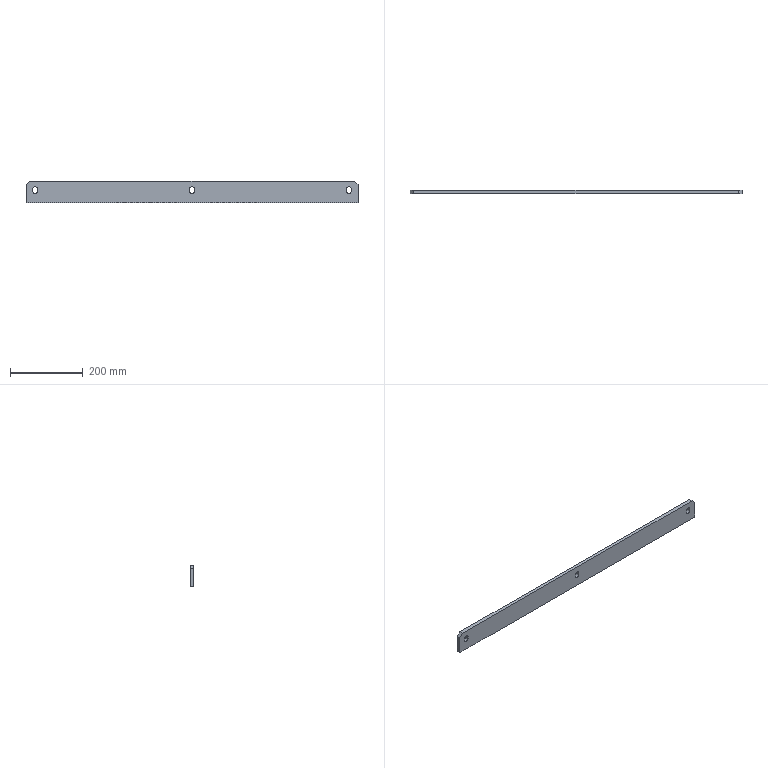Part | NX | features solid 2 | 1 solid | 20 faces | box 910 x 10 x 60 mm | volume 538678 mm3 | plane 14 | cylinder 6 | commonest cylinder face diameters 13 x6
STEP:
#1=CARTESIAN_POINT('',(570.,10.,-50.));
#2=VERTEX_POINT('',#1);
#3=CARTESIAN_POINT('',(580.,10.,-60.));
#4=VERTEX_POINT('',#3);
#5=CARTESIAN_POINT('',(580.,10.,-60.));
#6=DIRECTION('',(0.7071,0.,-0.7071));
#7=VECTOR('',#6,1000.);
#8=LINE('',#5,#7);
#9=EDGE_CURVE('',#2,#4,#8,.T.);
#10=ORIENTED_EDGE('',*,*,#9,.F.);
#11=CARTESIAN_POINT('',(570.,0.,-50.));
#12=VERTEX_POINT('',#11);
#13=CARTESIAN_POINT('',(570.,0.,-50.));
#14=DIRECTION('',(0.,1.,0.));
#15=VECTOR('',#14,1000.);
#16=LINE('',#13,#15);
#17=EDGE_CURVE('',#12,#2,#16,.T.);
#18=ORIENTED_EDGE('',*,*,#17,.F.);
#19=CARTESIAN_POINT('',(580.,0.,-60.));
#20=VERTEX_POINT('',#19);
#21=CARTESIAN_POINT('',(155.,0.,365.));
#22=DIRECTION('',(-0.7071,0.,0.7071));
#23=VECTOR('',#22,1000.);
#24=LINE('',#21,#23);
#25=EDGE_CURVE('',#20,#12,#24,.T.);
#26=ORIENTED_EDGE('',*,*,#25,.F.);
#27=CARTESIAN_POINT('',(580.,10.,-60.));
#28=DIRECTION('',(0.,-1.,0.));
#29=VECTOR('',#28,1000.);
#30=LINE('',#27,#29);
#31=EDGE_CURVE('',#4,#20,#30,.T.);
#32=ORIENTED_EDGE('',*,*,#31,.F.);
#33=EDGE_LOOP('',(#10,#18,#26,#32));
#34=FACE_BOUND('',#33,.T.);
#35=CARTESIAN_POINT('',(580.,10.,-60.));
#36=DIRECTION('',(-0.7071,0.,-0.7071));
#37=DIRECTION('',(-0.7071,0.,0.7071));
#38=AXIS2_PLACEMENT_3D('',#35,#36,#37);
#39=PLANE('',#38);
#40=ADVANCED_FACE('',(#34),#39,.F.);
#41=CARTESIAN_POINT('',(-330.,10.,-60.));
#42=VERTEX_POINT('',#41);
#43=CARTESIAN_POINT('',(-320.,10.,-50.));
#44=VERTEX_POINT('',#43);
#45=CARTESIAN_POINT('',(-320.,10.,-50.));
#46=DIRECTION('',(0.7071,0.,0.7071));
#47=VECTOR('',#46,1000.);
#48=LINE('',#45,#47);
#49=EDGE_CURVE('',#42,#44,#48,.T.);
#50=ORIENTED_EDGE('',*,*,#49,.F.);
#51=CARTESIAN_POINT('',(-330.,0.,-60.));
#52=VERTEX_POINT('',#51);
#53=CARTESIAN_POINT('',(-330.,10.,-60.));
#54=DIRECTION('',(0.,1.,0.));
#55=VECTOR('',#54,1000.);
#56=LINE('',#53,#55);
#57=EDGE_CURVE('',#52,#42,#56,.T.);
#58=ORIENTED_EDGE('',*,*,#57,.F.);
#59=CARTESIAN_POINT('',(-320.,0.,-50.));
#60=VERTEX_POINT('',#59);
#61=CARTESIAN_POINT('',(-360.,0.,-90.));
#62=DIRECTION('',(-0.7071,0.,-0.7071));
#63=VECTOR('',#62,1000.);
#64=LINE('',#61,#63);
#65=EDGE_CURVE('',#60,#52,#64,.T.);
#66=ORIENTED_EDGE('',*,*,#65,.F.);
#67=CARTESIAN_POINT('',(-320.,0.,-50.));
#68=DIRECTION('',(0.,-1.,0.));
#69=VECTOR('',#68,1000.);
#70=LINE('',#67,#69);
#71=EDGE_CURVE('',#44,#60,#70,.T.);
#72=ORIENTED_EDGE('',*,*,#71,.F.);
#73=EDGE_LOOP('',(#50,#58,#66,#72));
#74=FACE_BOUND('',#73,.T.);
#75=CARTESIAN_POINT('',(-320.,0.,-50.));
#76=DIRECTION('',(0.7071,0.,-0.7071));
#77=DIRECTION('',(0.,-1.,0.));
#78=AXIS2_PLACEMENT_3D('',#75,#76,#77);
#79=PLANE('',#78);
#80=ADVANCED_FACE('',(#74),#79,.F.);
#81=CARTESIAN_POINT('',(580.,10.,-110.));
#82=VERTEX_POINT('',#81);
#83=CARTESIAN_POINT('',(580.,10.,-120.));
#84=DIRECTION('',(0.,0.,1.));
#85=VECTOR('',#84,1000.);
#86=LINE('',#83,#85);
#87=EDGE_CURVE('',#82,#4,#86,.T.);
#88=ORIENTED_EDGE('',*,*,#87,.T.);
#89=ORIENTED_EDGE('',*,*,#31,.T.);
#90=CARTESIAN_POINT('',(580.,0.,-110.));
#91=VERTEX_POINT('',#90);
#92=CARTESIAN_POINT('',(580.,0.,-120.));
#93=DIRECTION('',(0.,0.,1.));
#94=VECTOR('',#93,1000.);
#95=LINE('',#92,#94);
#96=EDGE_CURVE('',#91,#20,#95,.T.);
#97=ORIENTED_EDGE('',*,*,#96,.F.);
#98=CARTESIAN_POINT('',(580.,10.,-110.));
#99=DIRECTION('',(0.,1.,0.));
#100=VECTOR('',#99,1000.);
#101=LINE('',#98,#100);
#102=EDGE_CURVE('',#91,#82,#101,.T.);
#103=ORIENTED_EDGE('',*,*,#102,.T.);
#104=EDGE_LOOP('',(#88,#89,#97,#103));
#105=FACE_BOUND('',#104,.T.);
#106=CARTESIAN_POINT('',(580.,10.,-120.));
#107=DIRECTION('',(-1.,0.,0.));
#108=DIRECTION('',(0.,0.,1.));
#109=AXIS2_PLACEMENT_3D('',#106,#107,#108);
#110=PLANE('',#109);
#111=ADVANCED_FACE('',(#105),#110,.F.);
#112=CARTESIAN_POINT('',(561.5,0.,-78.));
#113=VERTEX_POINT('',#112);
#114=CARTESIAN_POINT('',(561.5,10.,-78.));
#115=VERTEX_POINT('',#114);
#116=CARTESIAN_POINT('',(561.5,5.,-78.));
#117=DIRECTION('',(0.,1.,0.));
#118=VECTOR('',#117,1000.);
#119=LINE('',#116,#118);
#120=EDGE_CURVE('',#113,#115,#119,.T.);
#121=ORIENTED_EDGE('',*,*,#120,.T.);
#122=CARTESIAN_POINT('',(548.5,10.,-78.));
#123=VERTEX_POINT('',#122);
#124=CARTESIAN_POINT('',(555.,10.,-78.));
#125=DIRECTION('',(0.,1.,0.));
#126=DIRECTION('',(1.,0.,0.));
#127=AXIS2_PLACEMENT_3D('',#124,#125,#126);
#128=CIRCLE('',#127,6.5);
#129=EDGE_CURVE('',#115,#123,#128,.T.);
#130=ORIENTED_EDGE('',*,*,#129,.T.);
#131=CARTESIAN_POINT('',(548.5,0.,-78.));
#132=VERTEX_POINT('',#131);
#133=CARTESIAN_POINT('',(548.5,5.,-78.));
#134=DIRECTION('',(0.,-1.,0.));
#135=VECTOR('',#134,1000.);
#136=LINE('',#133,#135);
#137=EDGE_CURVE('',#123,#132,#136,.T.);
#138=ORIENTED_EDGE('',*,*,#137,.T.);
#139=CARTESIAN_POINT('',(555.,0.,-78.));
#140=DIRECTION('',(0.,1.,0.));
#141=DIRECTION('',(1.,0.,0.));
#142=AXIS2_PLACEMENT_3D('',#139,#140,#141);
#143=CIRCLE('',#142,6.5);
#144=EDGE_CURVE('',#113,#132,#143,.T.);
#145=ORIENTED_EDGE('',*,*,#144,.F.);
#146=EDGE_LOOP('',(#121,#130,#138,#145));
#147=FACE_BOUND('',#146,.T.);
#148=CARTESIAN_POINT('',(555.,5.,-78.));
#149=DIRECTION('',(0.,-1.,0.));
#150=DIRECTION('',(1.,0.,0.));
#151=AXIS2_PLACEMENT_3D('',#148,#149,#150);
#152=CYLINDRICAL_SURFACE('',#151,6.5);
#153=ADVANCED_FACE('',(#147),#152,.F.);
#154=ORIENTED_EDGE('',*,*,#137,.F.);
#155=CARTESIAN_POINT('',(548.5,10.,-72.));
#156=VERTEX_POINT('',#155);
#157=CARTESIAN_POINT('',(548.5,10.,-78.));
#158=DIRECTION('',(0.,0.,1.));
#159=VECTOR('',#158,1000.);
#160=LINE('',#157,#159);
#161=EDGE_CURVE('',#123,#156,#160,.T.);
#162=ORIENTED_EDGE('',*,*,#161,.T.);
#163=CARTESIAN_POINT('',(548.5,0.,-72.));
#164=VERTEX_POINT('',#163);
#165=CARTESIAN_POINT('',(548.5,10.,-72.));
#166=DIRECTION('',(0.,-1.,0.));
#167=VECTOR('',#166,1000.);
#168=LINE('',#165,#167);
#169=EDGE_CURVE('',#156,#164,#168,.T.);
#170=ORIENTED_EDGE('',*,*,#169,.T.);
#171=CARTESIAN_POINT('',(548.5,0.,-78.));
#172=DIRECTION('',(0.,0.,1.));
#173=VECTOR('',#172,1000.);
#174=LINE('',#171,#173);
#175=EDGE_CURVE('',#132,#164,#174,.T.);
#176=ORIENTED_EDGE('',*,*,#175,.F.);
#177=EDGE_LOOP('',(#154,#162,#170,#176));
#178=FACE_BOUND('',#177,.T.);
#179=CARTESIAN_POINT('',(548.5,10.,-78.));
#180=DIRECTION('',(-1.,0.,0.));
#181=DIRECTION('',(0.,0.,1.));
#182=AXIS2_PLACEMENT_3D('',#179,#180,#181);
#183=PLANE('',#182);
#184=ADVANCED_FACE('',(#178),#183,.F.);
#185=ORIENTED_EDGE('',*,*,#169,.F.);
#186=CARTESIAN_POINT('',(561.5,10.,-72.));
#187=VERTEX_POINT('',#186);
#188=CARTESIAN_POINT('',(555.,10.,-72.));
#189=DIRECTION('',(0.,1.,0.));
#190=DIRECTION('',(1.,0.,0.));
#191=AXIS2_PLACEMENT_3D('',#188,#189,#190);
#192=CIRCLE('',#191,6.5);
#193=EDGE_CURVE('',#156,#187,#192,.T.);
#194=ORIENTED_EDGE('',*,*,#193,.T.);
#195=CARTESIAN_POINT('',(561.5,0.,-72.));
#196=VERTEX_POINT('',#195);
#197=CARTESIAN_POINT('',(561.5,5.,-72.));
#198=DIRECTION('',(0.,-1.,0.));
#199=VECTOR('',#198,1000.);
#200=LINE('',#197,#199);
#201=EDGE_CURVE('',#187,#196,#200,.T.);
#202=ORIENTED_EDGE('',*,*,#201,.T.);
#203=CARTESIAN_POINT('',(555.,0.,-72.));
#204=DIRECTION('',(0.,1.,0.));
#205=DIRECTION('',(1.,0.,0.));
#206=AXIS2_PLACEMENT_3D('',#203,#204,#205);
#207=CIRCLE('',#206,6.5);
#208=EDGE_CURVE('',#164,#196,#207,.T.);
#209=ORIENTED_EDGE('',*,*,#208,.F.);
#210=EDGE_LOOP('',(#185,#194,#202,#209));
#211=FACE_BOUND('',#210,.T.);
#212=CARTESIAN_POINT('',(555.,5.,-72.));
#213=DIRECTION('',(0.,-1.,0.));
#214=DIRECTION('',(1.,0.,0.));
#215=AXIS2_PLACEMENT_3D('',#212,#213,#214);
#216=CYLINDRICAL_SURFACE('',#215,6.5);
#217=ADVANCED_FACE('',(#211),#216,.F.);
#218=ORIENTED_EDGE('',*,*,#201,.F.);
#219=CARTESIAN_POINT('',(561.5,10.,-78.));
#220=DIRECTION('',(0.,0.,-1.));
#221=VECTOR('',#220,1000.);
#222=LINE('',#219,#221);
#223=EDGE_CURVE('',#187,#115,#222,.T.);
#224=ORIENTED_EDGE('',*,*,#223,.T.);
#225=ORIENTED_EDGE('',*,*,#120,.F.);
#226=CARTESIAN_POINT('',(561.5,0.,-78.));
#227=DIRECTION('',(0.,0.,-1.));
#228=VECTOR('',#227,1000.);
#229=LINE('',#226,#228);
#230=EDGE_CURVE('',#196,#113,#229,.T.);
#231=ORIENTED_EDGE('',*,*,#230,.F.);
#232=EDGE_LOOP('',(#218,#224,#225,#231));
#233=FACE_BOUND('',#232,.T.);
#234=CARTESIAN_POINT('',(561.5,0.,-78.));
#235=DIRECTION('',(1.,0.,0.));
#236=DIRECTION('',(0.,-1.,0.));
#237=AXIS2_PLACEMENT_3D('',#234,#235,#236);
#238=PLANE('',#237);
#239=ADVANCED_FACE('',(#233),#238,.F.);
#240=CARTESIAN_POINT('',(131.5,0.,-78.));
#241=VERTEX_POINT('',#240);
#242=CARTESIAN_POINT('',(131.5,10.,-78.));
#243=VERTEX_POINT('',#242);
#244=CARTESIAN_POINT('',(131.5,5.,-78.));
#245=DIRECTION('',(0.,1.,0.));
#246=VECTOR('',#245,1000.);
#247=LINE('',#244,#246);
#248=EDGE_CURVE('',#241,#243,#247,.T.);
#249=ORIENTED_EDGE('',*,*,#248,.T.);
#250=CARTESIAN_POINT('',(118.5,10.,-78.));
#251=VERTEX_POINT('',#250);
#252=CARTESIAN_POINT('',(125.,10.,-78.));
#253=DIRECTION('',(0.,1.,0.));
#254=DIRECTION('',(1.,0.,0.));
#255=AXIS2_PLACEMENT_3D('',#252,#253,#254);
#256=CIRCLE('',#255,6.5);
#257=EDGE_CURVE('',#243,#251,#256,.T.);
#258=ORIENTED_EDGE('',*,*,#257,.T.);
#259=CARTESIAN_POINT('',(118.5,0.,-78.));
#260=VERTEX_POINT('',#259);
#261=CARTESIAN_POINT('',(118.5,5.,-78.));
#262=DIRECTION('',(0.,-1.,0.));
#263=VECTOR('',#262,1000.);
#264=LINE('',#261,#263);
#265=EDGE_CURVE('',#251,#260,#264,.T.);
#266=ORIENTED_EDGE('',*,*,#265,.T.);
#267=CARTESIAN_POINT('',(125.,0.,-78.));
#268=DIRECTION('',(0.,1.,0.));
#269=DIRECTION('',(1.,0.,0.));
#270=AXIS2_PLACEMENT_3D('',#267,#268,#269);
#271=CIRCLE('',#270,6.5);
#272=EDGE_CURVE('',#241,#260,#271,.T.);
#273=ORIENTED_EDGE('',*,*,#272,.F.);
#274=EDGE_LOOP('',(#249,#258,#266,#273));
#275=FACE_BOUND('',#274,.T.);
#276=CARTESIAN_POINT('',(125.,5.,-78.));
#277=DIRECTION('',(0.,-1.,0.));
#278=DIRECTION('',(1.,0.,0.));
#279=AXIS2_PLACEMENT_3D('',#276,#277,#278);
#280=CYLINDRICAL_SURFACE('',#279,6.5);
#281=ADVANCED_FACE('',(#275),#280,.F.);
#282=ORIENTED_EDGE('',*,*,#265,.F.);
#283=CARTESIAN_POINT('',(118.5,10.,-72.));
#284=VERTEX_POINT('',#283);
#285=CARTESIAN_POINT('',(118.5,10.,-78.));
#286=DIRECTION('',(0.,0.,1.));
#287=VECTOR('',#286,1000.);
#288=LINE('',#285,#287);
#289=EDGE_CURVE('',#251,#284,#288,.T.);
#290=ORIENTED_EDGE('',*,*,#289,.T.);
#291=CARTESIAN_POINT('',(118.5,0.,-72.));
#292=VERTEX_POINT('',#291);
#293=CARTESIAN_POINT('',(118.5,10.,-72.));
#294=DIRECTION('',(0.,-1.,0.));
#295=VECTOR('',#294,1000.);
#296=LINE('',#293,#295);
#297=EDGE_CURVE('',#284,#292,#296,.T.);
#298=ORIENTED_EDGE('',*,*,#297,.T.);
#299=CARTESIAN_POINT('',(118.5,0.,-78.));
#300=DIRECTION('',(0.,0.,1.));
#301=VECTOR('',#300,1000.);
#302=LINE('',#299,#301);
#303=EDGE_CURVE('',#260,#292,#302,.T.);
#304=ORIENTED_EDGE('',*,*,#303,.F.);
#305=EDGE_LOOP('',(#282,#290,#298,#304));
#306=FACE_BOUND('',#305,.T.);
#307=CARTESIAN_POINT('',(118.5,10.,-78.));
#308=DIRECTION('',(-1.,0.,0.));
#309=DIRECTION('',(0.,0.,1.));
#310=AXIS2_PLACEMENT_3D('',#307,#308,#309);
#311=PLANE('',#310);
#312=ADVANCED_FACE('',(#306),#311,.F.);
#313=ORIENTED_EDGE('',*,*,#297,.F.);
#314=CARTESIAN_POINT('',(131.5,10.,-72.));
#315=VERTEX_POINT('',#314);
#316=CARTESIAN_POINT('',(125.,10.,-72.));
#317=DIRECTION('',(0.,1.,0.));
#318=DIRECTION('',(1.,0.,0.));
#319=AXIS2_PLACEMENT_3D('',#316,#317,#318);
#320=CIRCLE('',#319,6.5);
#321=EDGE_CURVE('',#284,#315,#320,.T.);
#322=ORIENTED_EDGE('',*,*,#321,.T.);
#323=CARTESIAN_POINT('',(131.5,0.,-72.));
#324=VERTEX_POINT('',#323);
#325=CARTESIAN_POINT('',(131.5,5.,-72.));
#326=DIRECTION('',(0.,-1.,0.));
#327=VECTOR('',#326,1000.);
#328=LINE('',#325,#327);
#329=EDGE_CURVE('',#315,#324,#328,.T.);
#330=ORIENTED_EDGE('',*,*,#329,.T.);
#331=CARTESIAN_POINT('',(125.,0.,-72.));
#332=DIRECTION('',(0.,1.,0.));
#333=DIRECTION('',(1.,0.,0.));
#334=AXIS2_PLACEMENT_3D('',#331,#332,#333);
#335=CIRCLE('',#334,6.5);
#336=EDGE_CURVE('',#292,#324,#335,.T.);
#337=ORIENTED_EDGE('',*,*,#336,.F.);
#338=EDGE_LOOP('',(#313,#322,#330,#337));
#339=FACE_BOUND('',#338,.T.);
#340=CARTESIAN_POINT('',(125.,5.,-72.));
#341=DIRECTION('',(0.,-1.,0.));
#342=DIRECTION('',(1.,0.,0.));
#343=AXIS2_PLACEMENT_3D('',#340,#341,#342);
#344=CYLINDRICAL_SURFACE('',#343,6.5);
#345=ADVANCED_FACE('',(#339),#344,.F.);
#346=ORIENTED_EDGE('',*,*,#329,.F.);
#347=CARTESIAN_POINT('',(131.5,10.,-78.));
#348=DIRECTION('',(0.,0.,-1.));
#349=VECTOR('',#348,1000.);
#350=LINE('',#347,#349);
#351=EDGE_CURVE('',#315,#243,#350,.T.);
#352=ORIENTED_EDGE('',*,*,#351,.T.);
#353=ORIENTED_EDGE('',*,*,#248,.F.);
#354=CARTESIAN_POINT('',(131.5,0.,-78.));
#355=DIRECTION('',(0.,0.,-1.));
#356=VECTOR('',#355,1000.);
#357=LINE('',#354,#356);
#358=EDGE_CURVE('',#324,#241,#357,.T.);
#359=ORIENTED_EDGE('',*,*,#358,.F.);
#360=EDGE_LOOP('',(#346,#352,#353,#359));
#361=FACE_BOUND('',#360,.T.);
#362=CARTESIAN_POINT('',(131.5,0.,-78.));
#363=DIRECTION('',(1.,0.,0.));
#364=DIRECTION('',(0.,-1.,0.));
#365=AXIS2_PLACEMENT_3D('',#362,#363,#364);
#366=PLANE('',#365);
#367=ADVANCED_FACE('',(#361),#366,.F.);
#368=CARTESIAN_POINT('',(-298.5,0.,-78.));
#369=VERTEX_POINT('',#368);
#370=CARTESIAN_POINT('',(-298.5,10.,-78.));
#371=VERTEX_POINT('',#370);
#372=CARTESIAN_POINT('',(-298.5,5.,-78.));
#373=DIRECTION('',(0.,1.,0.));
#374=VECTOR('',#373,1000.);
#375=LINE('',#372,#374);
#376=EDGE_CURVE('',#369,#371,#375,.T.);
#377=ORIENTED_EDGE('',*,*,#376,.T.);
#378=CARTESIAN_POINT('',(-311.5,10.,-78.));
#379=VERTEX_POINT('',#378);
#380=CARTESIAN_POINT('',(-305.,10.,-78.));
#381=DIRECTION('',(0.,1.,0.));
#382=DIRECTION('',(1.,0.,0.));
#383=AXIS2_PLACEMENT_3D('',#380,#381,#382);
#384=CIRCLE('',#383,6.5);
#385=EDGE_CURVE('',#371,#379,#384,.T.);
#386=ORIENTED_EDGE('',*,*,#385,.T.);
#387=CARTESIAN_POINT('',(-311.5,0.,-78.));
#388=VERTEX_POINT('',#387);
#389=CARTESIAN_POINT('',(-311.5,5.,-78.));
#390=DIRECTION('',(0.,-1.,0.));
#391=VECTOR('',#390,1000.);
#392=LINE('',#389,#391);
#393=EDGE_CURVE('',#379,#388,#392,.T.);
#394=ORIENTED_EDGE('',*,*,#393,.T.);
#395=CARTESIAN_POINT('',(-305.,0.,-78.));
#396=DIRECTION('',(0.,1.,0.));
#397=DIRECTION('',(1.,0.,0.));
#398=AXIS2_PLACEMENT_3D('',#395,#396,#397);
#399=CIRCLE('',#398,6.5);
#400=EDGE_CURVE('',#369,#388,#399,.T.);
#401=ORIENTED_EDGE('',*,*,#400,.F.);
#402=EDGE_LOOP('',(#377,#386,#394,#401));
#403=FACE_BOUND('',#402,.T.);
#404=CARTESIAN_POINT('',(-305.,5.,-78.));
#405=DIRECTION('',(0.,-1.,0.));
#406=DIRECTION('',(1.,0.,0.));
#407=AXIS2_PLACEMENT_3D('',#404,#405,#406);
#408=CYLINDRICAL_SURFACE('',#407,6.5);
#409=ADVANCED_FACE('',(#403),#408,.F.);
#410=ORIENTED_EDGE('',*,*,#393,.F.);
#411=CARTESIAN_POINT('',(-311.5,10.,-72.));
#412=VERTEX_POINT('',#411);
#413=CARTESIAN_POINT('',(-311.5,10.,-78.));
#414=DIRECTION('',(0.,0.,1.));
#415=VECTOR('',#414,1000.);
#416=LINE('',#413,#415);
#417=EDGE_CURVE('',#379,#412,#416,.T.);
#418=ORIENTED_EDGE('',*,*,#417,.T.);
#419=CARTESIAN_POINT('',(-311.5,0.,-72.));
#420=VERTEX_POINT('',#419);
#421=CARTESIAN_POINT('',(-311.5,10.,-72.));
#422=DIRECTION('',(0.,-1.,0.));
#423=VECTOR('',#422,1000.);
#424=LINE('',#421,#423);
#425=EDGE_CURVE('',#412,#420,#424,.T.);
#426=ORIENTED_EDGE('',*,*,#425,.T.);
#427=CARTESIAN_POINT('',(-311.5,0.,-78.));
#428=DIRECTION('',(0.,0.,1.));
#429=VECTOR('',#428,1000.);
#430=LINE('',#427,#429);
#431=EDGE_CURVE('',#388,#420,#430,.T.);
#432=ORIENTED_EDGE('',*,*,#431,.F.);
#433=EDGE_LOOP('',(#410,#418,#426,#432));
#434=FACE_BOUND('',#433,.T.);
#435=CARTESIAN_POINT('',(-311.5,10.,-78.));
#436=DIRECTION('',(-1.,0.,0.));
#437=DIRECTION('',(0.,0.,1.));
#438=AXIS2_PLACEMENT_3D('',#435,#436,#437);
#439=PLANE('',#438);
#440=ADVANCED_FACE('',(#434),#439,.F.);
#441=ORIENTED_EDGE('',*,*,#425,.F.);
#442=CARTESIAN_POINT('',(-298.5,10.,-72.));
#443=VERTEX_POINT('',#442);
#444=CARTESIAN_POINT('',(-305.,10.,-72.));
#445=DIRECTION('',(0.,1.,0.));
#446=DIRECTION('',(1.,0.,0.));
#447=AXIS2_PLACEMENT_3D('',#444,#445,#446);
#448=CIRCLE('',#447,6.5);
#449=EDGE_CURVE('',#412,#443,#448,.T.);
#450=ORIENTED_EDGE('',*,*,#449,.T.);
#451=CARTESIAN_POINT('',(-298.5,0.,-72.));
#452=VERTEX_POINT('',#451);
#453=CARTESIAN_POINT('',(-298.5,5.,-72.));
#454=DIRECTION('',(0.,-1.,0.));
#455=VECTOR('',#454,1000.);
#456=LINE('',#453,#455);
#457=EDGE_CURVE('',#443,#452,#456,.T.);
#458=ORIENTED_EDGE('',*,*,#457,.T.);
#459=CARTESIAN_POINT('',(-305.,0.,-72.));
#460=DIRECTION('',(0.,1.,0.));
#461=DIRECTION('',(1.,0.,0.));
#462=AXIS2_PLACEMENT_3D('',#459,#460,#461);
#463=CIRCLE('',#462,6.5);
#464=EDGE_CURVE('',#420,#452,#463,.T.);
#465=ORIENTED_EDGE('',*,*,#464,.F.);
#466=EDGE_LOOP('',(#441,#450,#458,#465));
#467=FACE_BOUND('',#466,.T.);
#468=CARTESIAN_POINT('',(-305.,5.,-72.));
#469=DIRECTION('',(0.,-1.,0.));
#470=DIRECTION('',(1.,0.,0.));
#471=AXIS2_PLACEMENT_3D('',#468,#469,#470);
#472=CYLINDRICAL_SURFACE('',#471,6.5);
#473=ADVANCED_FACE('',(#467),#472,.F.);
#474=ORIENTED_EDGE('',*,*,#457,.F.);
#475=CARTESIAN_POINT('',(-298.5,10.,-78.));
#476=DIRECTION('',(0.,0.,-1.));
#477=VECTOR('',#476,1000.);
#478=LINE('',#475,#477);
#479=EDGE_CURVE('',#443,#371,#478,.T.);
#480=ORIENTED_EDGE('',*,*,#479,.T.);
#481=ORIENTED_EDGE('',*,*,#376,.F.);
#482=CARTESIAN_POINT('',(-298.5,0.,-78.));
#483=DIRECTION('',(0.,0.,-1.));
#484=VECTOR('',#483,1000.);
#485=LINE('',#482,#484);
#486=EDGE_CURVE('',#452,#369,#485,.T.);
#487=ORIENTED_EDGE('',*,*,#486,.F.);
#488=EDGE_LOOP('',(#474,#480,#481,#487));
#489=FACE_BOUND('',#488,.T.);
#490=CARTESIAN_POINT('',(-298.5,0.,-78.));
#491=DIRECTION('',(1.,0.,0.));
#492=DIRECTION('',(0.,-1.,0.));
#493=AXIS2_PLACEMENT_3D('',#490,#491,#492);
#494=PLANE('',#493);
#495=ADVANCED_FACE('',(#489),#494,.F.);
#496=CARTESIAN_POINT('',(-330.,10.,-50.));
#497=DIRECTION('',(-1.,0.,0.));
#498=VECTOR('',#497,1000.);
#499=LINE('',#496,#498);
#500=EDGE_CURVE('',#2,#44,#499,.T.);
#501=ORIENTED_EDGE('',*,*,#500,.T.);
#502=ORIENTED_EDGE('',*,*,#71,.T.);
#503=CARTESIAN_POINT('',(-330.,0.,-50.));
#504=DIRECTION('',(-1.,0.,0.));
#505=VECTOR('',#504,1000.);
#506=LINE('',#503,#505);
#507=EDGE_CURVE('',#12,#60,#506,.T.);
#508=ORIENTED_EDGE('',*,*,#507,.F.);
#509=ORIENTED_EDGE('',*,*,#17,.T.);
#510=EDGE_LOOP('',(#501,#502,#508,#509));
#511=FACE_BOUND('',#510,.T.);
#512=CARTESIAN_POINT('',(-330.,0.,-50.));
#513=DIRECTION('',(0.,0.,-1.));
#514=DIRECTION('',(-1.,0.,0.));
#515=AXIS2_PLACEMENT_3D('',#512,#513,#514);
#516=PLANE('',#515);
#517=ADVANCED_FACE('',(#511),#516,.F.);
#518=ORIENTED_EDGE('',*,*,#144,.T.);
#519=ORIENTED_EDGE('',*,*,#175,.T.);
#520=ORIENTED_EDGE('',*,*,#208,.T.);
#521=ORIENTED_EDGE('',*,*,#230,.T.);
#522=EDGE_LOOP('',(#518,#519,#520,#521));
#523=FACE_BOUND('',#522,.T.);
#524=ORIENTED_EDGE('',*,*,#272,.T.);
#525=ORIENTED_EDGE('',*,*,#303,.T.);
#526=ORIENTED_EDGE('',*,*,#336,.T.);
#527=ORIENTED_EDGE('',*,*,#358,.T.);
#528=EDGE_LOOP('',(#524,#525,#526,#527));
#529=FACE_BOUND('',#528,.T.);
#530=ORIENTED_EDGE('',*,*,#400,.T.);
#531=ORIENTED_EDGE('',*,*,#431,.T.);
#532=ORIENTED_EDGE('',*,*,#464,.T.);
#533=ORIENTED_EDGE('',*,*,#486,.T.);
#534=EDGE_LOOP('',(#530,#531,#532,#533));
#535=FACE_BOUND('',#534,.T.);
#536=ORIENTED_EDGE('',*,*,#507,.T.);
#537=ORIENTED_EDGE('',*,*,#65,.T.);
#538=CARTESIAN_POINT('',(-330.,0.,-110.));
#539=VERTEX_POINT('',#538);
#540=CARTESIAN_POINT('',(-330.,0.,-120.));
#541=DIRECTION('',(0.,0.,-1.));
#542=VECTOR('',#541,1000.);
#543=LINE('',#540,#542);
#544=EDGE_CURVE('',#52,#539,#543,.T.);
#545=ORIENTED_EDGE('',*,*,#544,.T.);
#546=CARTESIAN_POINT('',(610.,0.,-110.));
#547=DIRECTION('',(1.,0.,0.));
#548=VECTOR('',#547,1000.);
#549=LINE('',#546,#548);
#550=EDGE_CURVE('',#539,#91,#549,.T.);
#551=ORIENTED_EDGE('',*,*,#550,.T.);
#552=ORIENTED_EDGE('',*,*,#96,.T.);
#553=ORIENTED_EDGE('',*,*,#25,.T.);
#554=EDGE_LOOP('',(#536,#537,#545,#551,#552,#553));
#555=FACE_BOUND('',#554,.T.);
#556=CARTESIAN_POINT('',(-330.,0.,-120.));
#557=DIRECTION('',(0.,-1.,0.));
#558=DIRECTION('',(-1.,0.,0.));
#559=AXIS2_PLACEMENT_3D('',#556,#557,#558);
#560=PLANE('',#559);
#561=ADVANCED_FACE('',(#523,#529,#535,#555),#560,.T.);
#562=ORIENTED_EDGE('',*,*,#102,.F.);
#563=ORIENTED_EDGE('',*,*,#550,.F.);
#564=CARTESIAN_POINT('',(-330.,10.,-110.));
#565=VERTEX_POINT('',#564);
#566=CARTESIAN_POINT('',(-330.,10.,-110.));
#567=DIRECTION('',(0.,1.,0.));
#568=VECTOR('',#567,1000.);
#569=LINE('',#566,#568);
#570=EDGE_CURVE('',#539,#565,#569,.T.);
#571=ORIENTED_EDGE('',*,*,#570,.T.);
#572=CARTESIAN_POINT('',(610.,10.,-110.));
#573=DIRECTION('',(1.,0.,0.));
#574=VECTOR('',#573,1000.);
#575=LINE('',#572,#574);
#576=EDGE_CURVE('',#565,#82,#575,.T.);
#577=ORIENTED_EDGE('',*,*,#576,.T.);
#578=EDGE_LOOP('',(#562,#563,#571,#577));
#579=FACE_BOUND('',#578,.T.);
#580=CARTESIAN_POINT('',(610.,10.,-110.));
#581=DIRECTION('',(0.,0.,1.));
#582=DIRECTION('',(0.,-1.,0.));
#583=AXIS2_PLACEMENT_3D('',#580,#581,#582);
#584=PLANE('',#583);
#585=ADVANCED_FACE('',(#579),#584,.F.);
#586=ORIENTED_EDGE('',*,*,#193,.F.);
#587=ORIENTED_EDGE('',*,*,#161,.F.);
#588=ORIENTED_EDGE('',*,*,#129,.F.);
#589=ORIENTED_EDGE('',*,*,#223,.F.);
#590=EDGE_LOOP('',(#586,#587,#588,#589));
#591=FACE_BOUND('',#590,.T.);
#592=ORIENTED_EDGE('',*,*,#321,.F.);
#593=ORIENTED_EDGE('',*,*,#289,.F.);
#594=ORIENTED_EDGE('',*,*,#257,.F.);
#595=ORIENTED_EDGE('',*,*,#351,.F.);
#596=EDGE_LOOP('',(#592,#593,#594,#595));
#597=FACE_BOUND('',#596,.T.);
#598=ORIENTED_EDGE('',*,*,#449,.F.);
#599=ORIENTED_EDGE('',*,*,#417,.F.);
#600=ORIENTED_EDGE('',*,*,#385,.F.);
#601=ORIENTED_EDGE('',*,*,#479,.F.);
#602=EDGE_LOOP('',(#598,#599,#600,#601));
#603=FACE_BOUND('',#602,.T.);
#604=CARTESIAN_POINT('',(-330.,10.,-120.));
#605=DIRECTION('',(0.,0.,1.));
#606=VECTOR('',#605,1000.);
#607=LINE('',#604,#606);
#608=EDGE_CURVE('',#565,#42,#607,.T.);
#609=ORIENTED_EDGE('',*,*,#608,.T.);
#610=ORIENTED_EDGE('',*,*,#49,.T.);
#611=ORIENTED_EDGE('',*,*,#500,.F.);
#612=ORIENTED_EDGE('',*,*,#9,.T.);
#613=ORIENTED_EDGE('',*,*,#87,.F.);
#614=ORIENTED_EDGE('',*,*,#576,.F.);
#615=EDGE_LOOP('',(#609,#610,#611,#612,#613,#614));
#616=FACE_BOUND('',#615,.T.);
#617=CARTESIAN_POINT('',(-330.,10.,-120.));
#618=DIRECTION('',(0.,-1.,0.));
#619=DIRECTION('',(-1.,0.,0.));
#620=AXIS2_PLACEMENT_3D('',#617,#618,#619);
#621=PLANE('',#620);
#622=ADVANCED_FACE('',(#591,#597,#603,#616),#621,.F.);
#623=ORIENTED_EDGE('',*,*,#544,.F.);
#624=ORIENTED_EDGE('',*,*,#57,.T.);
#625=ORIENTED_EDGE('',*,*,#608,.F.);
#626=ORIENTED_EDGE('',*,*,#570,.F.);
#627=EDGE_LOOP('',(#623,#624,#625,#626));
#628=FACE_BOUND('',#627,.T.);
#629=CARTESIAN_POINT('',(-330.,10.,-120.));
#630=DIRECTION('',(1.,0.,0.));
#631=DIRECTION('',(0.,-1.,0.));
#632=AXIS2_PLACEMENT_3D('',#629,#630,#631);
#633=PLANE('',#632);
#634=ADVANCED_FACE('',(#628),#633,.F.);
#635=CLOSED_SHELL('',(#40,#80,#111,#153,#184,#217,#239,#281,#312,#345,#367,#409,#440,#473,#495,#517,#561,#585,#622,#634));
#636=MANIFOLD_SOLID_BREP('',#635);
#637=(LENGTH_UNIT()NAMED_UNIT(*)SI_UNIT(.MILLI.,.METRE.));
#638=UNCERTAINTY_MEASURE_WITH_UNIT(LENGTH_MEASURE(0.00001),#637,'','');
#639=(NAMED_UNIT(*)PLANE_ANGLE_UNIT()SI_UNIT($,.RADIAN.));
#640=(NAMED_UNIT(*)SI_UNIT($,.STERADIAN.)SOLID_ANGLE_UNIT());
#641=(GEOMETRIC_REPRESENTATION_CONTEXT(3)GLOBAL_UNCERTAINTY_ASSIGNED_CONTEXT((#638))GLOBAL_UNIT_ASSIGNED_CONTEXT((#637,#639,#640))REPRESENTATION_CONTEXT('',''));
#642=ADVANCED_BREP_SHAPE_REPRESENTATION('',(#636),#641);